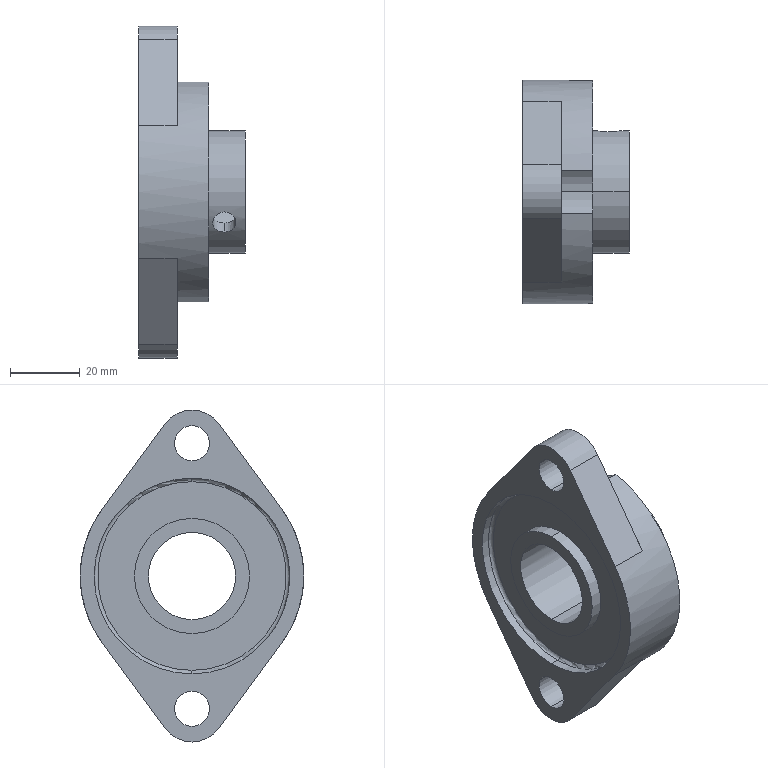Part | SolidWorks | features BaseBody 1 | 1 solid | 42 faces | box 30.5 x 64 x 95 mm | volume 54844 mm3 | cylinder 26 | plane 12 | torus 4 | commonest cylinder face diameters 6.647 x4 10 x4 56 x4 18 x3 19 x3 25 x2